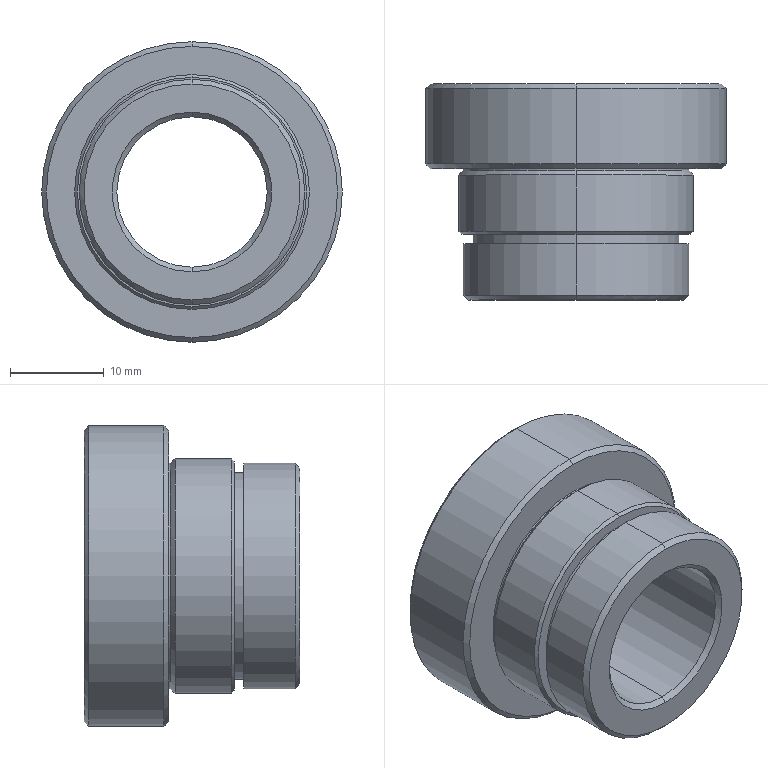Part | SolidWorks | features HoleWzd 1, Revolution 1 | 1 solid | 55 faces | box 32 x 23 x 32 mm | volume 8933 mm3 | cone 30 | cylinder 20 | plane 5 | commonest cylinder face diameters 2.5 x8 24 x4 16 x2 22 x2 25 x2 32 x2
STEP:
#1=CARTESIAN_POINT('',(-12.,-0.275,-1.25));
#2=VERTEX_POINT('',#1);
#3=CARTESIAN_POINT('',(-12.,-0.275,1.25));
#4=VERTEX_POINT('',#3);
#5=CARTESIAN_POINT('',(-12.,-0.275,0.));
#6=DIRECTION('',(0.,1.,0.));
#7=DIRECTION('',(0.,0.,1.));
#8=AXIS2_PLACEMENT_3D('',#5,#6,#7);
#9=CIRCLE('',#8,1.25);
#10=EDGE_CURVE('',#2,#4,#9,.T.);
#11=ORIENTED_EDGE('',*,*,#10,.F.);
#12=CARTESIAN_POINT('',(-12.,0.,-1.525));
#13=VERTEX_POINT('',#12);
#14=CARTESIAN_POINT('',(-12.,0.,-1.525));
#15=DIRECTION('',(0.,0.7071,-0.7071));
#16=VECTOR('',#15,1000.);
#17=LINE('',#14,#16);
#18=EDGE_CURVE('',#2,#13,#17,.T.);
#19=ORIENTED_EDGE('',*,*,#18,.T.);
#20=CARTESIAN_POINT('',(-12.,0.,1.525));
#21=VERTEX_POINT('',#20);
#22=CARTESIAN_POINT('',(-12.,0.,0.));
#23=DIRECTION('',(0.,1.,0.));
#24=DIRECTION('',(0.,0.,1.));
#25=AXIS2_PLACEMENT_3D('',#22,#23,#24);
#26=CIRCLE('',#25,1.525);
#27=EDGE_CURVE('',#13,#21,#26,.T.);
#28=ORIENTED_EDGE('',*,*,#27,.T.);
#29=CARTESIAN_POINT('',(-12.,0.,1.525));
#30=DIRECTION('',(0.,0.7071,0.7071));
#31=VECTOR('',#30,1000.);
#32=LINE('',#29,#31);
#33=EDGE_CURVE('',#4,#21,#32,.T.);
#34=ORIENTED_EDGE('',*,*,#33,.F.);
#35=EDGE_LOOP('',(#11,#19,#28,#34));
#36=FACE_OUTER_BOUND('',#35,.T.);
#37=CARTESIAN_POINT('',(-12.,0.,0.));
#38=DIRECTION('',(0.,1.,0.));
#39=DIRECTION('',(0.,0.,1.));
#40=AXIS2_PLACEMENT_3D('',#37,#38,#39);
#41=CONICAL_SURFACE('',#40,1.525,0.7854);
#42=ADVANCED_FACE('',(#36),#41,.F.);
#43=CARTESIAN_POINT('',(-12.,-7.,-1.25));
#44=VERTEX_POINT('',#43);
#45=CARTESIAN_POINT('',(-12.,-7.,1.25));
#46=VERTEX_POINT('',#45);
#47=CARTESIAN_POINT('',(-12.,-7.,0.));
#48=DIRECTION('',(0.,1.,0.));
#49=DIRECTION('',(0.,0.,1.));
#50=AXIS2_PLACEMENT_3D('',#47,#48,#49);
#51=CIRCLE('',#50,1.25);
#52=EDGE_CURVE('',#44,#46,#51,.T.);
#53=ORIENTED_EDGE('',*,*,#52,.F.);
#54=CARTESIAN_POINT('',(-12.,0.,-1.25));
#55=DIRECTION('',(0.,1.,0.));
#56=VECTOR('',#55,1000.);
#57=LINE('',#54,#56);
#58=EDGE_CURVE('',#44,#2,#57,.T.);
#59=ORIENTED_EDGE('',*,*,#58,.T.);
#60=ORIENTED_EDGE('',*,*,#10,.T.);
#61=CARTESIAN_POINT('',(-12.,0.,1.25));
#62=DIRECTION('',(0.,1.,0.));
#63=VECTOR('',#62,1000.);
#64=LINE('',#61,#63);
#65=EDGE_CURVE('',#46,#4,#64,.T.);
#66=ORIENTED_EDGE('',*,*,#65,.F.);
#67=EDGE_LOOP('',(#53,#59,#60,#66));
#68=FACE_OUTER_BOUND('',#67,.T.);
#69=CARTESIAN_POINT('',(-12.,0.,0.));
#70=DIRECTION('',(0.,1.,0.));
#71=DIRECTION('',(0.,0.,1.));
#72=AXIS2_PLACEMENT_3D('',#69,#70,#71);
#73=CYLINDRICAL_SURFACE('',#72,1.25);
#74=ADVANCED_FACE('',(#68),#73,.F.);
#75=CARTESIAN_POINT('',(-12.,-7.751,0.));
#76=VERTEX_POINT('',#75);
#77=CARTESIAN_POINT('',(-12.,-7.,1.25));
#78=DIRECTION('',(0.,0.515,0.8572));
#79=VECTOR('',#78,1000.);
#80=LINE('',#77,#79);
#81=EDGE_CURVE('',#76,#46,#80,.T.);
#82=ORIENTED_EDGE('',*,*,#81,.F.);
#83=CARTESIAN_POINT('',(-12.,-7.,-1.25));
#84=DIRECTION('',(0.,0.515,-0.8572));
#85=VECTOR('',#84,1000.);
#86=LINE('',#83,#85);
#87=EDGE_CURVE('',#76,#44,#86,.T.);
#88=ORIENTED_EDGE('',*,*,#87,.T.);
#89=ORIENTED_EDGE('',*,*,#52,.T.);
#90=EDGE_LOOP('',(#82,#88,#89));
#91=FACE_OUTER_BOUND('',#90,.T.);
#92=CARTESIAN_POINT('',(-12.,-7.,0.));
#93=DIRECTION('',(0.,1.,0.));
#94=DIRECTION('',(0.,0.,1.));
#95=AXIS2_PLACEMENT_3D('',#92,#93,#94);
#96=CONICAL_SURFACE('',#95,1.25,1.03);
#97=ADVANCED_FACE('',(#91),#96,.F.);
#98=CARTESIAN_POINT('',(0.,-0.275,-13.25));
#99=VERTEX_POINT('',#98);
#100=CARTESIAN_POINT('',(0.,-0.275,-10.75));
#101=VERTEX_POINT('',#100);
#102=CARTESIAN_POINT('',(0.,-0.275,-12.));
#103=DIRECTION('',(0.,1.,0.));
#104=DIRECTION('',(0.,0.,1.));
#105=AXIS2_PLACEMENT_3D('',#102,#103,#104);
#106=CIRCLE('',#105,1.25);
#107=EDGE_CURVE('',#99,#101,#106,.T.);
#108=ORIENTED_EDGE('',*,*,#107,.F.);
#109=CARTESIAN_POINT('',(0.,0.,-13.525));
#110=VERTEX_POINT('',#109);
#111=CARTESIAN_POINT('',(0.,0.,-13.525));
#112=DIRECTION('',(0.,0.7071,-0.7071));
#113=VECTOR('',#112,1000.);
#114=LINE('',#111,#113);
#115=EDGE_CURVE('',#99,#110,#114,.T.);
#116=ORIENTED_EDGE('',*,*,#115,.T.);
#117=CARTESIAN_POINT('',(0.,0.,-10.475));
#118=VERTEX_POINT('',#117);
#119=CARTESIAN_POINT('',(0.,0.,-12.));
#120=DIRECTION('',(0.,1.,0.));
#121=DIRECTION('',(0.,0.,1.));
#122=AXIS2_PLACEMENT_3D('',#119,#120,#121);
#123=CIRCLE('',#122,1.525);
#124=EDGE_CURVE('',#110,#118,#123,.T.);
#125=ORIENTED_EDGE('',*,*,#124,.T.);
#126=CARTESIAN_POINT('',(0.,0.,-10.475));
#127=DIRECTION('',(0.,0.7071,0.7071));
#128=VECTOR('',#127,1000.);
#129=LINE('',#126,#128);
#130=EDGE_CURVE('',#101,#118,#129,.T.);
#131=ORIENTED_EDGE('',*,*,#130,.F.);
#132=EDGE_LOOP('',(#108,#116,#125,#131));
#133=FACE_OUTER_BOUND('',#132,.T.);
#134=CARTESIAN_POINT('',(0.,0.,-12.));
#135=DIRECTION('',(0.,1.,0.));
#136=DIRECTION('',(0.,0.,1.));
#137=AXIS2_PLACEMENT_3D('',#134,#135,#136);
#138=CONICAL_SURFACE('',#137,1.525,0.7854);
#139=ADVANCED_FACE('',(#133),#138,.F.);
#140=CARTESIAN_POINT('',(0.,-7.,-13.25));
#141=VERTEX_POINT('',#140);
#142=CARTESIAN_POINT('',(0.,-7.,-10.75));
#143=VERTEX_POINT('',#142);
#144=CARTESIAN_POINT('',(0.,-7.,-12.));
#145=DIRECTION('',(0.,1.,0.));
#146=DIRECTION('',(0.,0.,1.));
#147=AXIS2_PLACEMENT_3D('',#144,#145,#146);
#148=CIRCLE('',#147,1.25);
#149=EDGE_CURVE('',#141,#143,#148,.T.);
#150=ORIENTED_EDGE('',*,*,#149,.F.);
#151=CARTESIAN_POINT('',(0.,0.,-13.25));
#152=DIRECTION('',(0.,1.,0.));
#153=VECTOR('',#152,1000.);
#154=LINE('',#151,#153);
#155=EDGE_CURVE('',#141,#99,#154,.T.);
#156=ORIENTED_EDGE('',*,*,#155,.T.);
#157=ORIENTED_EDGE('',*,*,#107,.T.);
#158=CARTESIAN_POINT('',(0.,0.,-10.75));
#159=DIRECTION('',(0.,1.,0.));
#160=VECTOR('',#159,1000.);
#161=LINE('',#158,#160);
#162=EDGE_CURVE('',#143,#101,#161,.T.);
#163=ORIENTED_EDGE('',*,*,#162,.F.);
#164=EDGE_LOOP('',(#150,#156,#157,#163));
#165=FACE_OUTER_BOUND('',#164,.T.);
#166=CARTESIAN_POINT('',(0.,0.,-12.));
#167=DIRECTION('',(0.,1.,0.));
#168=DIRECTION('',(0.,0.,1.));
#169=AXIS2_PLACEMENT_3D('',#166,#167,#168);
#170=CYLINDRICAL_SURFACE('',#169,1.25);
#171=ADVANCED_FACE('',(#165),#170,.F.);
#172=CARTESIAN_POINT('',(0.,-7.751,-12.));
#173=VERTEX_POINT('',#172);
#174=CARTESIAN_POINT('',(0.,-7.,-10.75));
#175=DIRECTION('',(0.,0.515,0.8572));
#176=VECTOR('',#175,1000.);
#177=LINE('',#174,#176);
#178=EDGE_CURVE('',#173,#143,#177,.T.);
#179=ORIENTED_EDGE('',*,*,#178,.F.);
#180=CARTESIAN_POINT('',(0.,-7.,-13.25));
#181=DIRECTION('',(0.,0.515,-0.8572));
#182=VECTOR('',#181,1000.);
#183=LINE('',#180,#182);
#184=EDGE_CURVE('',#173,#141,#183,.T.);
#185=ORIENTED_EDGE('',*,*,#184,.T.);
#186=ORIENTED_EDGE('',*,*,#149,.T.);
#187=EDGE_LOOP('',(#179,#185,#186));
#188=FACE_OUTER_BOUND('',#187,.T.);
#189=CARTESIAN_POINT('',(0.,-7.,-12.));
#190=DIRECTION('',(0.,1.,0.));
#191=DIRECTION('',(0.,0.,1.));
#192=AXIS2_PLACEMENT_3D('',#189,#190,#191);
#193=CONICAL_SURFACE('',#192,1.25,1.03);
#194=ADVANCED_FACE('',(#188),#193,.F.);
#195=CARTESIAN_POINT('',(12.,-0.275,-1.25));
#196=VERTEX_POINT('',#195);
#197=CARTESIAN_POINT('',(12.,-0.275,1.25));
#198=VERTEX_POINT('',#197);
#199=CARTESIAN_POINT('',(12.,-0.275,0.));
#200=DIRECTION('',(0.,1.,0.));
#201=DIRECTION('',(0.,0.,1.));
#202=AXIS2_PLACEMENT_3D('',#199,#200,#201);
#203=CIRCLE('',#202,1.25);
#204=EDGE_CURVE('',#196,#198,#203,.T.);
#205=ORIENTED_EDGE('',*,*,#204,.F.);
#206=CARTESIAN_POINT('',(12.,0.,-1.525));
#207=VERTEX_POINT('',#206);
#208=CARTESIAN_POINT('',(12.,0.,-1.525));
#209=DIRECTION('',(0.,0.7071,-0.7071));
#210=VECTOR('',#209,1000.);
#211=LINE('',#208,#210);
#212=EDGE_CURVE('',#196,#207,#211,.T.);
#213=ORIENTED_EDGE('',*,*,#212,.T.);
#214=CARTESIAN_POINT('',(12.,0.,1.525));
#215=VERTEX_POINT('',#214);
#216=CARTESIAN_POINT('',(12.,0.,0.));
#217=DIRECTION('',(0.,1.,0.));
#218=DIRECTION('',(0.,0.,1.));
#219=AXIS2_PLACEMENT_3D('',#216,#217,#218);
#220=CIRCLE('',#219,1.525);
#221=EDGE_CURVE('',#207,#215,#220,.T.);
#222=ORIENTED_EDGE('',*,*,#221,.T.);
#223=CARTESIAN_POINT('',(12.,0.,1.525));
#224=DIRECTION('',(0.,0.7071,0.7071));
#225=VECTOR('',#224,1000.);
#226=LINE('',#223,#225);
#227=EDGE_CURVE('',#198,#215,#226,.T.);
#228=ORIENTED_EDGE('',*,*,#227,.F.);
#229=EDGE_LOOP('',(#205,#213,#222,#228));
#230=FACE_OUTER_BOUND('',#229,.T.);
#231=CARTESIAN_POINT('',(12.,0.,0.));
#232=DIRECTION('',(0.,1.,0.));
#233=DIRECTION('',(0.,0.,1.));
#234=AXIS2_PLACEMENT_3D('',#231,#232,#233);
#235=CONICAL_SURFACE('',#234,1.525,0.7854);
#236=ADVANCED_FACE('',(#230),#235,.F.);
#237=CARTESIAN_POINT('',(12.,-7.,-1.25));
#238=VERTEX_POINT('',#237);
#239=CARTESIAN_POINT('',(12.,-7.,1.25));
#240=VERTEX_POINT('',#239);
#241=CARTESIAN_POINT('',(12.,-7.,0.));
#242=DIRECTION('',(0.,1.,0.));
#243=DIRECTION('',(0.,0.,1.));
#244=AXIS2_PLACEMENT_3D('',#241,#242,#243);
#245=CIRCLE('',#244,1.25);
#246=EDGE_CURVE('',#238,#240,#245,.T.);
#247=ORIENTED_EDGE('',*,*,#246,.F.);
#248=CARTESIAN_POINT('',(12.,0.,-1.25));
#249=DIRECTION('',(0.,1.,0.));
#250=VECTOR('',#249,1000.);
#251=LINE('',#248,#250);
#252=EDGE_CURVE('',#238,#196,#251,.T.);
#253=ORIENTED_EDGE('',*,*,#252,.T.);
#254=ORIENTED_EDGE('',*,*,#204,.T.);
#255=CARTESIAN_POINT('',(12.,0.,1.25));
#256=DIRECTION('',(0.,1.,0.));
#257=VECTOR('',#256,1000.);
#258=LINE('',#255,#257);
#259=EDGE_CURVE('',#240,#198,#258,.T.);
#260=ORIENTED_EDGE('',*,*,#259,.F.);
#261=EDGE_LOOP('',(#247,#253,#254,#260));
#262=FACE_OUTER_BOUND('',#261,.T.);
#263=CARTESIAN_POINT('',(12.,0.,0.));
#264=DIRECTION('',(0.,1.,0.));
#265=DIRECTION('',(0.,0.,1.));
#266=AXIS2_PLACEMENT_3D('',#263,#264,#265);
#267=CYLINDRICAL_SURFACE('',#266,1.25);
#268=ADVANCED_FACE('',(#262),#267,.F.);
#269=CARTESIAN_POINT('',(12.,-7.751,0.));
#270=VERTEX_POINT('',#269);
#271=CARTESIAN_POINT('',(12.,-7.,1.25));
#272=DIRECTION('',(0.,0.515,0.8572));
#273=VECTOR('',#272,1000.);
#274=LINE('',#271,#273);
#275=EDGE_CURVE('',#270,#240,#274,.T.);
#276=ORIENTED_EDGE('',*,*,#275,.F.);
#277=CARTESIAN_POINT('',(12.,-7.,-1.25));
#278=DIRECTION('',(0.,0.515,-0.8572));
#279=VECTOR('',#278,1000.);
#280=LINE('',#277,#279);
#281=EDGE_CURVE('',#270,#238,#280,.T.);
#282=ORIENTED_EDGE('',*,*,#281,.T.);
#283=ORIENTED_EDGE('',*,*,#246,.T.);
#284=EDGE_LOOP('',(#276,#282,#283));
#285=FACE_OUTER_BOUND('',#284,.T.);
#286=CARTESIAN_POINT('',(12.,-7.,0.));
#287=DIRECTION('',(0.,1.,0.));
#288=DIRECTION('',(0.,0.,1.));
#289=AXIS2_PLACEMENT_3D('',#286,#287,#288);
#290=CONICAL_SURFACE('',#289,1.25,1.03);
#291=ADVANCED_FACE('',(#285),#290,.F.);
#292=CARTESIAN_POINT('',(0.,-0.275,10.75));
#293=VERTEX_POINT('',#292);
#294=CARTESIAN_POINT('',(0.,-0.275,13.25));
#295=VERTEX_POINT('',#294);
#296=CARTESIAN_POINT('',(0.,-0.275,12.));
#297=DIRECTION('',(0.,1.,0.));
#298=DIRECTION('',(0.,0.,1.));
#299=AXIS2_PLACEMENT_3D('',#296,#297,#298);
#300=CIRCLE('',#299,1.25);
#301=EDGE_CURVE('',#293,#295,#300,.T.);
#302=ORIENTED_EDGE('',*,*,#301,.F.);
#303=CARTESIAN_POINT('',(0.,0.,10.475));
#304=VERTEX_POINT('',#303);
#305=CARTESIAN_POINT('',(0.,0.,10.475));
#306=DIRECTION('',(0.,0.7071,-0.7071));
#307=VECTOR('',#306,1000.);
#308=LINE('',#305,#307);
#309=EDGE_CURVE('',#293,#304,#308,.T.);
#310=ORIENTED_EDGE('',*,*,#309,.T.);
#311=CARTESIAN_POINT('',(0.,0.,13.525));
#312=VERTEX_POINT('',#311);
#313=CARTESIAN_POINT('',(0.,0.,12.));
#314=DIRECTION('',(0.,1.,0.));
#315=DIRECTION('',(0.,0.,1.));
#316=AXIS2_PLACEMENT_3D('',#313,#314,#315);
#317=CIRCLE('',#316,1.525);
#318=EDGE_CURVE('',#304,#312,#317,.T.);
#319=ORIENTED_EDGE('',*,*,#318,.T.);
#320=CARTESIAN_POINT('',(0.,0.,13.525));
#321=DIRECTION('',(0.,0.7071,0.7071));
#322=VECTOR('',#321,1000.);
#323=LINE('',#320,#322);
#324=EDGE_CURVE('',#295,#312,#323,.T.);
#325=ORIENTED_EDGE('',*,*,#324,.F.);
#326=EDGE_LOOP('',(#302,#310,#319,#325));
#327=FACE_OUTER_BOUND('',#326,.T.);
#328=CARTESIAN_POINT('',(0.,0.,12.));
#329=DIRECTION('',(0.,1.,0.));
#330=DIRECTION('',(0.,0.,1.));
#331=AXIS2_PLACEMENT_3D('',#328,#329,#330);
#332=CONICAL_SURFACE('',#331,1.525,0.7854);
#333=ADVANCED_FACE('',(#327),#332,.F.);
#334=CARTESIAN_POINT('',(0.,-7.,10.75));
#335=VERTEX_POINT('',#334);
#336=CARTESIAN_POINT('',(0.,-7.,13.25));
#337=VERTEX_POINT('',#336);
#338=CARTESIAN_POINT('',(0.,-7.,12.));
#339=DIRECTION('',(0.,1.,0.));
#340=DIRECTION('',(0.,0.,1.));
#341=AXIS2_PLACEMENT_3D('',#338,#339,#340);
#342=CIRCLE('',#341,1.25);
#343=EDGE_CURVE('',#335,#337,#342,.T.);
#344=ORIENTED_EDGE('',*,*,#343,.F.);
#345=CARTESIAN_POINT('',(0.,0.,10.75));
#346=DIRECTION('',(0.,1.,0.));
#347=VECTOR('',#346,1000.);
#348=LINE('',#345,#347);
#349=EDGE_CURVE('',#335,#293,#348,.T.);
#350=ORIENTED_EDGE('',*,*,#349,.T.);
#351=ORIENTED_EDGE('',*,*,#301,.T.);
#352=CARTESIAN_POINT('',(0.,0.,13.25));
#353=DIRECTION('',(0.,1.,0.));
#354=VECTOR('',#353,1000.);
#355=LINE('',#352,#354);
#356=EDGE_CURVE('',#337,#295,#355,.T.);
#357=ORIENTED_EDGE('',*,*,#356,.F.);
#358=EDGE_LOOP('',(#344,#350,#351,#357));
#359=FACE_OUTER_BOUND('',#358,.T.);
#360=CARTESIAN_POINT('',(0.,0.,12.));
#361=DIRECTION('',(0.,1.,0.));
#362=DIRECTION('',(0.,0.,1.));
#363=AXIS2_PLACEMENT_3D('',#360,#361,#362);
#364=CYLINDRICAL_SURFACE('',#363,1.25);
#365=ADVANCED_FACE('',(#359),#364,.F.);
#366=CARTESIAN_POINT('',(0.,-7.751,12.));
#367=VERTEX_POINT('',#366);
#368=CARTESIAN_POINT('',(0.,-7.,13.25));
#369=DIRECTION('',(0.,0.515,0.8572));
#370=VECTOR('',#369,1000.);
#371=LINE('',#368,#370);
#372=EDGE_CURVE('',#367,#337,#371,.T.);
#373=ORIENTED_EDGE('',*,*,#372,.F.);
#374=CARTESIAN_POINT('',(0.,-7.,10.75));
#375=DIRECTION('',(0.,0.515,-0.8572));
#376=VECTOR('',#375,1000.);
#377=LINE('',#374,#376);
#378=EDGE_CURVE('',#367,#335,#377,.T.);
#379=ORIENTED_EDGE('',*,*,#378,.T.);
#380=ORIENTED_EDGE('',*,*,#343,.T.);
#381=EDGE_LOOP('',(#373,#379,#380));
#382=FACE_OUTER_BOUND('',#381,.T.);
#383=CARTESIAN_POINT('',(0.,-7.,12.));
#384=DIRECTION('',(0.,1.,0.));
#385=DIRECTION('',(0.,0.,1.));
#386=AXIS2_PLACEMENT_3D('',#383,#384,#385);
#387=CONICAL_SURFACE('',#386,1.25,1.03);
#388=ADVANCED_FACE('',(#382),#387,.F.);
#389=CARTESIAN_POINT('',(0.,-22.5,-8.));
#390=VERTEX_POINT('',#389);
#391=CARTESIAN_POINT('',(0.,-22.5,8.));
#392=VERTEX_POINT('',#391);
#393=CARTESIAN_POINT('',(0.,-22.5,0.));
#394=DIRECTION('',(0.,1.,0.));
#395=DIRECTION('',(0.,0.,1.));
#396=AXIS2_PLACEMENT_3D('',#393,#394,#395);
#397=CIRCLE('',#396,8.);
#398=EDGE_CURVE('',#390,#392,#397,.T.);
#399=ORIENTED_EDGE('',*,*,#398,.F.);
#400=CARTESIAN_POINT('',(0.,-0.5,-8.));
#401=VERTEX_POINT('',#400);
#402=CARTESIAN_POINT('',(0.,0.,-8.));
#403=DIRECTION('',(0.,1.,0.));
#404=VECTOR('',#403,1000.);
#405=LINE('',#402,#404);
#406=EDGE_CURVE('',#390,#401,#405,.T.);
#407=ORIENTED_EDGE('',*,*,#406,.T.);
#408=CARTESIAN_POINT('',(0.,-0.5,8.));
#409=VERTEX_POINT('',#408);
#410=CARTESIAN_POINT('',(0.,-0.5,0.));
#411=DIRECTION('',(0.,1.,0.));
#412=DIRECTION('',(0.,0.,1.));
#413=AXIS2_PLACEMENT_3D('',#410,#411,#412);
#414=CIRCLE('',#413,8.);
#415=EDGE_CURVE('',#401,#409,#414,.T.);
#416=ORIENTED_EDGE('',*,*,#415,.T.);
#417=CARTESIAN_POINT('',(0.,0.,8.));
#418=DIRECTION('',(0.,1.,0.));
#419=VECTOR('',#418,1000.);
#420=LINE('',#417,#419);
#421=EDGE_CURVE('',#392,#409,#420,.T.);
#422=ORIENTED_EDGE('',*,*,#421,.F.);
#423=EDGE_LOOP('',(#399,#407,#416,#422));
#424=FACE_OUTER_BOUND('',#423,.T.);
#425=CARTESIAN_POINT('',(0.,0.,0.));
#426=DIRECTION('',(0.,1.,0.));
#427=DIRECTION('',(0.,0.,1.));
#428=AXIS2_PLACEMENT_3D('',#425,#426,#427);
#429=CYLINDRICAL_SURFACE('',#428,8.);
#430=ADVANCED_FACE('',(#424),#429,.F.);
#431=ORIENTED_EDGE('',*,*,#415,.F.);
#432=CARTESIAN_POINT('',(0.,0.,-8.5));
#433=VERTEX_POINT('',#432);
#434=CARTESIAN_POINT('',(0.,0.,-8.5));
#435=DIRECTION('',(0.,0.7071,-0.7071));
#436=VECTOR('',#435,1000.);
#437=LINE('',#434,#436);
#438=EDGE_CURVE('',#401,#433,#437,.T.);
#439=ORIENTED_EDGE('',*,*,#438,.T.);
#440=CARTESIAN_POINT('',(0.,0.,8.5));
#441=VERTEX_POINT('',#440);
#442=CARTESIAN_POINT('',(0.,0.,0.));
#443=DIRECTION('',(0.,1.,0.));
#444=DIRECTION('',(0.,0.,1.));
#445=AXIS2_PLACEMENT_3D('',#442,#443,#444);
#446=CIRCLE('',#445,8.5);
#447=EDGE_CURVE('',#433,#441,#446,.T.);
#448=ORIENTED_EDGE('',*,*,#447,.T.);
#449=CARTESIAN_POINT('',(0.,0.,8.5));
#450=DIRECTION('',(0.,0.7071,0.7071));
#451=VECTOR('',#450,1000.);
#452=LINE('',#449,#451);
#453=EDGE_CURVE('',#409,#441,#452,.T.);
#454=ORIENTED_EDGE('',*,*,#453,.F.);
#455=EDGE_LOOP('',(#431,#439,#448,#454));
#456=FACE_OUTER_BOUND('',#455,.T.);
#457=CARTESIAN_POINT('',(0.,0.,0.));
#458=DIRECTION('',(0.,1.,0.));
#459=DIRECTION('',(0.,0.,1.));
#460=AXIS2_PLACEMENT_3D('',#457,#458,#459);
#461=CONICAL_SURFACE('',#460,8.5,0.7854);
#462=ADVANCED_FACE('',(#456),#461,.F.);
#463=CARTESIAN_POINT('',(0.,0.,15.5));
#464=VERTEX_POINT('',#463);
#465=CARTESIAN_POINT('',(0.,0.,-15.5));
#466=VERTEX_POINT('',#465);
#467=CARTESIAN_POINT('',(0.,0.,0.));
#468=DIRECTION('',(0.,1.,0.));
#469=DIRECTION('',(0.,0.,1.));
#470=AXIS2_PLACEMENT_3D('',#467,#468,#469);
#471=CIRCLE('',#470,15.5);
#472=EDGE_CURVE('',#464,#466,#471,.T.);
#473=ORIENTED_EDGE('',*,*,#472,.F.);
#474=CARTESIAN_POINT('',(0.,-0.5,16.));
#475=VERTEX_POINT('',#474);
#476=CARTESIAN_POINT('',(0.,-0.5,16.));
#477=DIRECTION('',(0.,-0.7071,0.7071));
#478=VECTOR('',#477,1000.);
#479=LINE('',#476,#478);
#480=EDGE_CURVE('',#464,#475,#479,.T.);
#481=ORIENTED_EDGE('',*,*,#480,.T.);
#482=CARTESIAN_POINT('',(0.,-0.5,-16.));
#483=VERTEX_POINT('',#482);
#484=CARTESIAN_POINT('',(0.,-0.5,0.));
#485=DIRECTION('',(0.,1.,0.));
#486=DIRECTION('',(0.,0.,1.));
#487=AXIS2_PLACEMENT_3D('',#484,#485,#486);
#488=CIRCLE('',#487,16.);
#489=EDGE_CURVE('',#475,#483,#488,.T.);
#490=ORIENTED_EDGE('',*,*,#489,.T.);
#491=CARTESIAN_POINT('',(0.,-0.5,-16.));
#492=DIRECTION('',(0.,-0.7071,-0.7071));
#493=VECTOR('',#492,1000.);
#494=LINE('',#491,#493);
#495=EDGE_CURVE('',#466,#483,#494,.T.);
#496=ORIENTED_EDGE('',*,*,#495,.F.);
#497=EDGE_LOOP('',(#473,#481,#490,#496));
#498=FACE_OUTER_BOUND('',#497,.T.);
#499=CARTESIAN_POINT('',(0.,-0.5,0.));
#500=DIRECTION('',(0.,-1.,0.));
#501=DIRECTION('',(0.,0.,-1.));
#502=AXIS2_PLACEMENT_3D('',#499,#500,#501);
#503=CONICAL_SURFACE('',#502,16.,0.7854);
#504=ADVANCED_FACE('',(#498),#503,.T.);
#505=CARTESIAN_POINT('',(0.,-8.5,16.));
#506=VERTEX_POINT('',#505);
#507=CARTESIAN_POINT('',(0.,-8.5,-16.));
#508=VERTEX_POINT('',#507);
#509=CARTESIAN_POINT('',(0.,-8.5,0.));
#510=DIRECTION('',(0.,1.,0.));
#511=DIRECTION('',(0.,0.,1.));
#512=AXIS2_PLACEMENT_3D('',#509,#510,#511);
#513=CIRCLE('',#512,16.);
#514=EDGE_CURVE('',#506,#508,#513,.T.);
#515=ORIENTED_EDGE('',*,*,#514,.T.);
#516=CARTESIAN_POINT('',(0.,0.,-16.));
#517=DIRECTION('',(0.,1.,0.));
#518=VECTOR('',#517,1000.);
#519=LINE('',#516,#518);
#520=EDGE_CURVE('',#508,#483,#519,.T.);
#521=ORIENTED_EDGE('',*,*,#520,.T.);
#522=ORIENTED_EDGE('',*,*,#489,.F.);
#523=CARTESIAN_POINT('',(0.,0.,16.));
#524=DIRECTION('',(0.,1.,0.));
#525=VECTOR('',#524,1000.);
#526=LINE('',#523,#525);
#527=EDGE_CURVE('',#506,#475,#526,.T.);
#528=ORIENTED_EDGE('',*,*,#527,.F.);
#529=EDGE_LOOP('',(#515,#521,#522,#528));
#530=FACE_OUTER_BOUND('',#529,.T.);
#531=CARTESIAN_POINT('',(0.,0.,0.));
#532=DIRECTION('',(0.,1.,0.));
#533=DIRECTION('',(0.,0.,1.));
#534=AXIS2_PLACEMENT_3D('',#531,#532,#533);
#535=CYLINDRICAL_SURFACE('',#534,16.);
#536=ADVANCED_FACE('',(#530),#535,.T.);
#537=CARTESIAN_POINT('',(0.,-9.,15.5));
#538=VERTEX_POINT('',#537);
#539=CARTESIAN_POINT('',(0.,-9.,-15.5));
#540=VERTEX_POINT('',#539);
#541=CARTESIAN_POINT('',(0.,-9.,0.));
#542=DIRECTION('',(0.,1.,0.));
#543=DIRECTION('',(0.,0.,1.));
#544=AXIS2_PLACEMENT_3D('',#541,#542,#543);
#545=CIRCLE('',#544,15.5);
#546=EDGE_CURVE('',#538,#540,#545,.T.);
#547=ORIENTED_EDGE('',*,*,#546,.T.);
#548=CARTESIAN_POINT('',(0.,-9.,-15.5));
#549=DIRECTION('',(0.,0.7071,-0.7071));
#550=VECTOR('',#549,1000.);
#551=LINE('',#548,#550);
#552=EDGE_CURVE('',#540,#508,#551,.T.);
#553=ORIENTED_EDGE('',*,*,#552,.T.);
#554=ORIENTED_EDGE('',*,*,#514,.F.);
#555=CARTESIAN_POINT('',(0.,-9.,15.5));
#556=DIRECTION('',(0.,0.7071,0.7071));
#557=VECTOR('',#556,1000.);
#558=LINE('',#555,#557);
#559=EDGE_CURVE('',#538,#506,#558,.T.);
#560=ORIENTED_EDGE('',*,*,#559,.F.);
#561=EDGE_LOOP('',(#547,#553,#554,#560));
#562=FACE_OUTER_BOUND('',#561,.T.);
#563=CARTESIAN_POINT('',(0.,-9.,0.));
#564=DIRECTION('',(0.,1.,0.));
#565=DIRECTION('',(0.,0.,1.));
#566=AXIS2_PLACEMENT_3D('',#563,#564,#565);
#567=CONICAL_SURFACE('',#566,15.5,0.7854);
#568=ADVANCED_FACE('',(#562),#567,.T.);
#569=CARTESIAN_POINT('',(0.,-9.2,12.));
#570=VERTEX_POINT('',#569);
#571=CARTESIAN_POINT('',(0.,-9.2,-12.));
#572=VERTEX_POINT('',#571);
#573=CARTESIAN_POINT('',(0.,-9.2,0.));
#574=DIRECTION('',(0.,1.,0.));
#575=DIRECTION('',(0.,0.,1.));
#576=AXIS2_PLACEMENT_3D('',#573,#574,#575);
#577=CIRCLE('',#576,12.);
#578=EDGE_CURVE('',#570,#572,#577,.T.);
#579=ORIENTED_EDGE('',*,*,#578,.T.);
#580=CARTESIAN_POINT('',(0.,-9.,-12.));
#581=VERTEX_POINT('',#580);
#582=CARTESIAN_POINT('',(0.,0.,-12.));
#583=DIRECTION('',(0.,1.,0.));
#584=VECTOR('',#583,1000.);
#585=LINE('',#582,#584);
#586=EDGE_CURVE('',#572,#581,#585,.T.);
#587=ORIENTED_EDGE('',*,*,#586,.T.);
#588=CARTESIAN_POINT('',(0.,-9.,12.));
#589=VERTEX_POINT('',#588);
#590=CARTESIAN_POINT('',(0.,-9.,0.));
#591=DIRECTION('',(0.,1.,0.));
#592=DIRECTION('',(0.,0.,1.));
#593=AXIS2_PLACEMENT_3D('',#590,#591,#592);
#594=CIRCLE('',#593,12.);
#595=EDGE_CURVE('',#589,#581,#594,.T.);
#596=ORIENTED_EDGE('',*,*,#595,.F.);
#597=CARTESIAN_POINT('',(0.,0.,12.));
#598=DIRECTION('',(0.,1.,0.));
#599=VECTOR('',#598,1000.);
#600=LINE('',#597,#599);
#601=EDGE_CURVE('',#570,#589,#600,.T.);
#602=ORIENTED_EDGE('',*,*,#601,.F.);
#603=EDGE_LOOP('',(#579,#587,#596,#602));
#604=FACE_OUTER_BOUND('',#603,.T.);
#605=CARTESIAN_POINT('',(0.,0.,0.));
#606=DIRECTION('',(0.,1.,0.));
#607=DIRECTION('',(0.,0.,1.));
#608=AXIS2_PLACEMENT_3D('',#605,#606,#607);
#609=CYLINDRICAL_SURFACE('',#608,12.);
#610=ADVANCED_FACE('',(#604),#609,.T.);
#611=ORIENTED_EDGE('',*,*,#578,.F.);
#612=CARTESIAN_POINT('',(0.,-9.7,12.5));
#613=VERTEX_POINT('',#612);
#614=CARTESIAN_POINT('',(0.,-9.7,12.5));
#615=DIRECTION('',(0.,-0.7071,0.7071));
#616=VECTOR('',#615,1000.);
#617=LINE('',#614,#616);
#618=EDGE_CURVE('',#570,#613,#617,.T.);
#619=ORIENTED_EDGE('',*,*,#618,.T.);
#620=CARTESIAN_POINT('',(0.,-9.7,-12.5));
#621=VERTEX_POINT('',#620);
#622=CARTESIAN_POINT('',(0.,-9.7,0.));
#623=DIRECTION('',(0.,1.,0.));
#624=DIRECTION('',(0.,0.,1.));
#625=AXIS2_PLACEMENT_3D('',#622,#623,#624);
#626=CIRCLE('',#625,12.5);
#627=EDGE_CURVE('',#613,#621,#626,.T.);
#628=ORIENTED_EDGE('',*,*,#627,.T.);
#629=CARTESIAN_POINT('',(0.,-9.7,-12.5));
#630=DIRECTION('',(0.,-0.7071,-0.7071));
#631=VECTOR('',#630,1000.);
#632=LINE('',#629,#631);
#633=EDGE_CURVE('',#572,#621,#632,.T.);
#634=ORIENTED_EDGE('',*,*,#633,.F.);
#635=EDGE_LOOP('',(#611,#619,#628,#634));
#636=FACE_OUTER_BOUND('',#635,.T.);
#637=CARTESIAN_POINT('',(0.,-9.7,0.));
#638=DIRECTION('',(0.,-1.,0.));
#639=DIRECTION('',(0.,0.,-1.));
#640=AXIS2_PLACEMENT_3D('',#637,#638,#639);
#641=CONICAL_SURFACE('',#640,12.5,0.7854);
#642=ADVANCED_FACE('',(#636),#641,.T.);
#643=CARTESIAN_POINT('',(0.,-15.7,12.5));
#644=VERTEX_POINT('',#643);
#645=CARTESIAN_POINT('',(0.,-15.7,-12.5));
#646=VERTEX_POINT('',#645);
#647=CARTESIAN_POINT('',(0.,-15.7,0.));
#648=DIRECTION('',(0.,1.,0.));
#649=DIRECTION('',(0.,0.,1.));
#650=AXIS2_PLACEMENT_3D('',#647,#648,#649);
#651=CIRCLE('',#650,12.5);
#652=EDGE_CURVE('',#644,#646,#651,.T.);
#653=ORIENTED_EDGE('',*,*,#652,.T.);
#654=CARTESIAN_POINT('',(0.,0.,-12.5));
#655=DIRECTION('',(0.,1.,0.));
#656=VECTOR('',#655,1000.);
#657=LINE('',#654,#656);
#658=EDGE_CURVE('',#646,#621,#657,.T.);
#659=ORIENTED_EDGE('',*,*,#658,.T.);
#660=ORIENTED_EDGE('',*,*,#627,.F.);
#661=CARTESIAN_POINT('',(0.,0.,12.5));
#662=DIRECTION('',(0.,1.,0.));
#663=VECTOR('',#662,1000.);
#664=LINE('',#661,#663);
#665=EDGE_CURVE('',#644,#613,#664,.T.);
#666=ORIENTED_EDGE('',*,*,#665,.F.);
#667=EDGE_LOOP('',(#653,#659,#660,#666));
#668=FACE_OUTER_BOUND('',#667,.T.);
#669=CARTESIAN_POINT('',(0.,0.,0.));
#670=DIRECTION('',(0.,1.,0.));
#671=DIRECTION('',(0.,0.,1.));
#672=AXIS2_PLACEMENT_3D('',#669,#670,#671);
#673=CYLINDRICAL_SURFACE('',#672,12.5);
#674=ADVANCED_FACE('',(#668),#673,.T.);
#675=CARTESIAN_POINT('',(0.,-16.,12.2));
#676=VERTEX_POINT('',#675);
#677=CARTESIAN_POINT('',(0.,-16.,-12.2));
#678=VERTEX_POINT('',#677);
#679=CARTESIAN_POINT('',(0.,-16.,0.));
#680=DIRECTION('',(0.,1.,0.));
#681=DIRECTION('',(0.,0.,1.));
#682=AXIS2_PLACEMENT_3D('',#679,#680,#681);
#683=CIRCLE('',#682,12.2);
#684=EDGE_CURVE('',#676,#678,#683,.T.);
#685=ORIENTED_EDGE('',*,*,#684,.T.);
#686=CARTESIAN_POINT('',(0.,-16.,-12.2));
#687=DIRECTION('',(0.,0.7071,-0.7071));
#688=VECTOR('',#687,1000.);
#689=LINE('',#686,#688);
#690=EDGE_CURVE('',#678,#646,#689,.T.);
#691=ORIENTED_EDGE('',*,*,#690,.T.);
#692=ORIENTED_EDGE('',*,*,#652,.F.);
#693=CARTESIAN_POINT('',(0.,-16.,12.2));
#694=DIRECTION('',(0.,0.7071,0.7071));
#695=VECTOR('',#694,1000.);
#696=LINE('',#693,#695);
#697=EDGE_CURVE('',#676,#644,#696,.T.);
#698=ORIENTED_EDGE('',*,*,#697,.F.);
#699=EDGE_LOOP('',(#685,#691,#692,#698));
#700=FACE_OUTER_BOUND('',#699,.T.);
#701=CARTESIAN_POINT('',(0.,-16.,0.));
#702=DIRECTION('',(0.,1.,0.));
#703=DIRECTION('',(0.,0.,1.));
#704=AXIS2_PLACEMENT_3D('',#701,#702,#703);
#705=CONICAL_SURFACE('',#704,12.2,0.7854);
#706=ADVANCED_FACE('',(#700),#705,.T.);
#707=CARTESIAN_POINT('',(0.,-17.,11.));
#708=VERTEX_POINT('',#707);
#709=CARTESIAN_POINT('',(0.,-17.,-11.));
#710=VERTEX_POINT('',#709);
#711=CARTESIAN_POINT('',(0.,-17.,0.));
#712=DIRECTION('',(0.,1.,0.));
#713=DIRECTION('',(0.,0.,1.));
#714=AXIS2_PLACEMENT_3D('',#711,#712,#713);
#715=CIRCLE('',#714,11.);
#716=EDGE_CURVE('',#708,#710,#715,.T.);
#717=ORIENTED_EDGE('',*,*,#716,.T.);
#718=CARTESIAN_POINT('',(0.,-16.,-11.));
#719=VERTEX_POINT('',#718);
#720=CARTESIAN_POINT('',(0.,0.,-11.));
#721=DIRECTION('',(0.,1.,0.));
#722=VECTOR('',#721,1000.);
#723=LINE('',#720,#722);
#724=EDGE_CURVE('',#710,#719,#723,.T.);
#725=ORIENTED_EDGE('',*,*,#724,.T.);
#726=CARTESIAN_POINT('',(0.,-16.,11.));
#727=VERTEX_POINT('',#726);
#728=CARTESIAN_POINT('',(0.,-16.,0.));
#729=DIRECTION('',(0.,1.,0.));
#730=DIRECTION('',(0.,0.,1.));
#731=AXIS2_PLACEMENT_3D('',#728,#729,#730);
#732=CIRCLE('',#731,11.);
#733=EDGE_CURVE('',#727,#719,#732,.T.);
#734=ORIENTED_EDGE('',*,*,#733,.F.);
#735=CARTESIAN_POINT('',(0.,0.,11.));
#736=DIRECTION('',(0.,1.,0.));
#737=VECTOR('',#736,1000.);
#738=LINE('',#735,#737);
#739=EDGE_CURVE('',#708,#727,#738,.T.);
#740=ORIENTED_EDGE('',*,*,#739,.F.);
#741=EDGE_LOOP('',(#717,#725,#734,#740));
#742=FACE_OUTER_BOUND('',#741,.T.);
#743=CARTESIAN_POINT('',(0.,0.,0.));
#744=DIRECTION('',(0.,1.,0.));
#745=DIRECTION('',(0.,0.,1.));
#746=AXIS2_PLACEMENT_3D('',#743,#744,#745);
#747=CYLINDRICAL_SURFACE('',#746,11.);
#748=ADVANCED_FACE('',(#742),#747,.T.);
#749=CARTESIAN_POINT('',(0.,-22.5,12.));
#750=VERTEX_POINT('',#749);
#751=CARTESIAN_POINT('',(0.,-22.5,-12.));
#752=VERTEX_POINT('',#751);
#753=CARTESIAN_POINT('',(0.,-22.5,0.));
#754=DIRECTION('',(0.,1.,0.));
#755=DIRECTION('',(0.,0.,1.));
#756=AXIS2_PLACEMENT_3D('',#753,#754,#755);
#757=CIRCLE('',#756,12.);
#758=EDGE_CURVE('',#750,#752,#757,.T.);
#759=ORIENTED_EDGE('',*,*,#758,.T.);
#760=CARTESIAN_POINT('',(0.,-17.,-12.));
#761=VERTEX_POINT('',#760);
#762=CARTESIAN_POINT('',(0.,0.,-12.));
#763=DIRECTION('',(0.,1.,0.));
#764=VECTOR('',#763,1000.);
#765=LINE('',#762,#764);
#766=EDGE_CURVE('',#752,#761,#765,.T.);
#767=ORIENTED_EDGE('',*,*,#766,.T.);
#768=CARTESIAN_POINT('',(0.,-17.,12.));
#769=VERTEX_POINT('',#768);
#770=CARTESIAN_POINT('',(0.,-17.,0.));
#771=DIRECTION('',(0.,1.,0.));
#772=DIRECTION('',(0.,0.,1.));
#773=AXIS2_PLACEMENT_3D('',#770,#771,#772);
#774=CIRCLE('',#773,12.);
#775=EDGE_CURVE('',#769,#761,#774,.T.);
#776=ORIENTED_EDGE('',*,*,#775,.F.);
#777=CARTESIAN_POINT('',(0.,0.,12.));
#778=DIRECTION('',(0.,1.,0.));
#779=VECTOR('',#778,1000.);
#780=LINE('',#777,#779);
#781=EDGE_CURVE('',#750,#769,#780,.T.);
#782=ORIENTED_EDGE('',*,*,#781,.F.);
#783=EDGE_LOOP('',(#759,#767,#776,#782));
#784=FACE_OUTER_BOUND('',#783,.T.);
#785=CARTESIAN_POINT('',(0.,0.,0.));
#786=DIRECTION('',(0.,1.,0.));
#787=DIRECTION('',(0.,0.,1.));
#788=AXIS2_PLACEMENT_3D('',#785,#786,#787);
#789=CYLINDRICAL_SURFACE('',#788,12.);
#790=ADVANCED_FACE('',(#784),#789,.T.);
#791=CARTESIAN_POINT('',(0.,-23.,11.5));
#792=VERTEX_POINT('',#791);
#793=CARTESIAN_POINT('',(0.,-23.,-11.5));
#794=VERTEX_POINT('',#793);
#795=CARTESIAN_POINT('',(0.,-23.,0.));
#796=DIRECTION('',(0.,1.,0.));
#797=DIRECTION('',(0.,0.,1.));
#798=AXIS2_PLACEMENT_3D('',#795,#796,#797);
#799=CIRCLE('',#798,11.5);
#800=EDGE_CURVE('',#792,#794,#799,.T.);
#801=ORIENTED_EDGE('',*,*,#800,.T.);
#802=CARTESIAN_POINT('',(0.,-23.,-11.5));
#803=DIRECTION('',(0.,0.7071,-0.7071));
#804=VECTOR('',#803,1000.);
#805=LINE('',#802,#804);
#806=EDGE_CURVE('',#794,#752,#805,.T.);
#807=ORIENTED_EDGE('',*,*,#806,.T.);
#808=ORIENTED_EDGE('',*,*,#758,.F.);
#809=CARTESIAN_POINT('',(0.,-23.,11.5));
#810=DIRECTION('',(0.,0.7071,0.7071));
#811=VECTOR('',#810,1000.);
#812=LINE('',#809,#811);
#813=EDGE_CURVE('',#792,#750,#812,.T.);
#814=ORIENTED_EDGE('',*,*,#813,.F.);
#815=EDGE_LOOP('',(#801,#807,#808,#814));
#816=FACE_OUTER_BOUND('',#815,.T.);
#817=CARTESIAN_POINT('',(0.,-23.,0.));
#818=DIRECTION('',(0.,1.,0.));
#819=DIRECTION('',(0.,0.,1.));
#820=AXIS2_PLACEMENT_3D('',#817,#818,#819);
#821=CONICAL_SURFACE('',#820,11.5,0.7854);
#822=ADVANCED_FACE('',(#816),#821,.T.);
#823=ORIENTED_EDGE('',*,*,#398,.T.);
#824=CARTESIAN_POINT('',(0.,-23.,8.5));
#825=VERTEX_POINT('',#824);
#826=CARTESIAN_POINT('',(0.,-22.5,8.));
#827=DIRECTION('',(0.,-0.7071,0.7071));
#828=VECTOR('',#827,1000.);
#829=LINE('',#826,#828);
#830=EDGE_CURVE('',#392,#825,#829,.T.);
#831=ORIENTED_EDGE('',*,*,#830,.T.);
#832=CARTESIAN_POINT('',(0.,-23.,-8.5));
#833=VERTEX_POINT('',#832);
#834=CARTESIAN_POINT('',(0.,-23.,0.));
#835=DIRECTION('',(0.,1.,0.));
#836=DIRECTION('',(0.,0.,1.));
#837=AXIS2_PLACEMENT_3D('',#834,#835,#836);
#838=CIRCLE('',#837,8.5);
#839=EDGE_CURVE('',#833,#825,#838,.T.);
#840=ORIENTED_EDGE('',*,*,#839,.F.);
#841=CARTESIAN_POINT('',(0.,-22.5,-8.));
#842=DIRECTION('',(0.,-0.7071,-0.7071));
#843=VECTOR('',#842,1000.);
#844=LINE('',#841,#843);
#845=EDGE_CURVE('',#390,#833,#844,.T.);
#846=ORIENTED_EDGE('',*,*,#845,.F.);
#847=EDGE_LOOP('',(#823,#831,#840,#846));
#848=FACE_OUTER_BOUND('',#847,.T.);
#849=CARTESIAN_POINT('',(0.,-22.5,0.));
#850=DIRECTION('',(0.,-1.,0.));
#851=DIRECTION('',(0.,0.,-1.));
#852=AXIS2_PLACEMENT_3D('',#849,#850,#851);
#853=CONICAL_SURFACE('',#852,8.,0.7854);
#854=ADVANCED_FACE('',(#848),#853,.F.);
#855=ORIENTED_EDGE('',*,*,#830,.F.);
#856=CARTESIAN_POINT('',(0.,-22.5,0.));
#857=DIRECTION('',(0.,1.,0.));
#858=DIRECTION('',(0.,0.,1.));
#859=AXIS2_PLACEMENT_3D('',#856,#857,#858);
#860=CIRCLE('',#859,8.);
#861=EDGE_CURVE('',#392,#390,#860,.T.);
#862=ORIENTED_EDGE('',*,*,#861,.T.);
#863=ORIENTED_EDGE('',*,*,#845,.T.);
#864=CARTESIAN_POINT('',(0.,-23.,0.));
#865=DIRECTION('',(0.,1.,0.));
#866=DIRECTION('',(0.,0.,1.));
#867=AXIS2_PLACEMENT_3D('',#864,#865,#866);
#868=CIRCLE('',#867,8.5);
#869=EDGE_CURVE('',#825,#833,#868,.T.);
#870=ORIENTED_EDGE('',*,*,#869,.F.);
#871=EDGE_LOOP('',(#855,#862,#863,#870));
#872=FACE_OUTER_BOUND('',#871,.T.);
#873=CARTESIAN_POINT('',(0.,-22.5,0.));
#874=DIRECTION('',(0.,-1.,0.));
#875=DIRECTION('',(0.,0.,-1.));
#876=AXIS2_PLACEMENT_3D('',#873,#874,#875);
#877=CONICAL_SURFACE('',#876,8.,0.7854);
#878=ADVANCED_FACE('',(#872),#877,.F.);
#879=ORIENTED_EDGE('',*,*,#800,.F.);
#880=CARTESIAN_POINT('',(0.,-23.,0.));
#881=DIRECTION('',(0.,1.,0.));
#882=DIRECTION('',(0.,0.,1.));
#883=AXIS2_PLACEMENT_3D('',#880,#881,#882);
#884=CIRCLE('',#883,11.5);
#885=EDGE_CURVE('',#794,#792,#884,.T.);
#886=ORIENTED_EDGE('',*,*,#885,.F.);
#887=EDGE_LOOP('',(#879,#886));
#888=FACE_OUTER_BOUND('',#887,.T.);
#889=ORIENTED_EDGE('',*,*,#839,.T.);
#890=ORIENTED_EDGE('',*,*,#869,.T.);
#891=EDGE_LOOP('',(#889,#890));
#892=FACE_BOUND('',#891,.T.);
#893=CARTESIAN_POINT('',(8.5,-23.,0.));
#894=DIRECTION('',(0.,1.,0.));
#895=DIRECTION('',(0.,0.,1.));
#896=AXIS2_PLACEMENT_3D('',#893,#894,#895);
#897=PLANE('',#896);
#898=ADVANCED_FACE('',(#888,#892),#897,.F.);
#899=ORIENTED_EDGE('',*,*,#806,.F.);
#900=ORIENTED_EDGE('',*,*,#885,.T.);
#901=ORIENTED_EDGE('',*,*,#813,.T.);
#902=CARTESIAN_POINT('',(0.,-22.5,0.));
#903=DIRECTION('',(0.,1.,0.));
#904=DIRECTION('',(0.,0.,1.));
#905=AXIS2_PLACEMENT_3D('',#902,#903,#904);
#906=CIRCLE('',#905,12.);
#907=EDGE_CURVE('',#752,#750,#906,.T.);
#908=ORIENTED_EDGE('',*,*,#907,.F.);
#909=EDGE_LOOP('',(#899,#900,#901,#908));
#910=FACE_OUTER_BOUND('',#909,.T.);
#911=CARTESIAN_POINT('',(0.,-23.,0.));
#912=DIRECTION('',(0.,1.,0.));
#913=DIRECTION('',(0.,0.,1.));
#914=AXIS2_PLACEMENT_3D('',#911,#912,#913);
#915=CONICAL_SURFACE('',#914,11.5,0.7854);
#916=ADVANCED_FACE('',(#910),#915,.T.);
#917=ORIENTED_EDGE('',*,*,#766,.F.);
#918=ORIENTED_EDGE('',*,*,#907,.T.);
#919=ORIENTED_EDGE('',*,*,#781,.T.);
#920=CARTESIAN_POINT('',(0.,-17.,0.));
#921=DIRECTION('',(0.,1.,0.));
#922=DIRECTION('',(0.,0.,1.));
#923=AXIS2_PLACEMENT_3D('',#920,#921,#922);
#924=CIRCLE('',#923,12.);
#925=EDGE_CURVE('',#761,#769,#924,.T.);
#926=ORIENTED_EDGE('',*,*,#925,.F.);
#927=EDGE_LOOP('',(#917,#918,#919,#926));
#928=FACE_OUTER_BOUND('',#927,.T.);
#929=CARTESIAN_POINT('',(0.,0.,0.));
#930=DIRECTION('',(0.,1.,0.));
#931=DIRECTION('',(0.,0.,1.));
#932=AXIS2_PLACEMENT_3D('',#929,#930,#931);
#933=CYLINDRICAL_SURFACE('',#932,12.);
#934=ADVANCED_FACE('',(#928),#933,.T.);
#935=ORIENTED_EDGE('',*,*,#716,.F.);
#936=CARTESIAN_POINT('',(0.,-17.,0.));
#937=DIRECTION('',(0.,1.,0.));
#938=DIRECTION('',(0.,0.,1.));
#939=AXIS2_PLACEMENT_3D('',#936,#937,#938);
#940=CIRCLE('',#939,11.);
#941=EDGE_CURVE('',#710,#708,#940,.T.);
#942=ORIENTED_EDGE('',*,*,#941,.F.);
#943=EDGE_LOOP('',(#935,#942));
#944=FACE_BOUND('',#943,.T.);
#945=ORIENTED_EDGE('',*,*,#775,.T.);
#946=ORIENTED_EDGE('',*,*,#925,.T.);
#947=EDGE_LOOP('',(#945,#946));
#948=FACE_OUTER_BOUND('',#947,.T.);
#949=CARTESIAN_POINT('',(11.,-17.,0.));
#950=DIRECTION('',(0.,-1.,0.));
#951=DIRECTION('',(0.,0.,-1.));
#952=AXIS2_PLACEMENT_3D('',#949,#950,#951);
#953=PLANE('',#952);
#954=ADVANCED_FACE('',(#944,#948),#953,.F.);
#955=ORIENTED_EDGE('',*,*,#724,.F.);
#956=ORIENTED_EDGE('',*,*,#941,.T.);
#957=ORIENTED_EDGE('',*,*,#739,.T.);
#958=CARTESIAN_POINT('',(0.,-16.,0.));
#959=DIRECTION('',(0.,1.,0.));
#960=DIRECTION('',(0.,0.,1.));
#961=AXIS2_PLACEMENT_3D('',#958,#959,#960);
#962=CIRCLE('',#961,11.);
#963=EDGE_CURVE('',#719,#727,#962,.T.);
#964=ORIENTED_EDGE('',*,*,#963,.F.);
#965=EDGE_LOOP('',(#955,#956,#957,#964));
#966=FACE_OUTER_BOUND('',#965,.T.);
#967=CARTESIAN_POINT('',(0.,0.,0.));
#968=DIRECTION('',(0.,1.,0.));
#969=DIRECTION('',(0.,0.,1.));
#970=AXIS2_PLACEMENT_3D('',#967,#968,#969);
#971=CYLINDRICAL_SURFACE('',#970,11.);
#972=ADVANCED_FACE('',(#966),#971,.T.);
#973=ORIENTED_EDGE('',*,*,#684,.F.);
#974=CARTESIAN_POINT('',(0.,-16.,0.));
#975=DIRECTION('',(0.,1.,0.));
#976=DIRECTION('',(0.,0.,1.));
#977=AXIS2_PLACEMENT_3D('',#974,#975,#976);
#978=CIRCLE('',#977,12.2);
#979=EDGE_CURVE('',#678,#676,#978,.T.);
#980=ORIENTED_EDGE('',*,*,#979,.F.);
#981=EDGE_LOOP('',(#973,#980));
#982=FACE_OUTER_BOUND('',#981,.T.);
#983=ORIENTED_EDGE('',*,*,#733,.T.);
#984=ORIENTED_EDGE('',*,*,#963,.T.);
#985=EDGE_LOOP('',(#983,#984));
#986=FACE_BOUND('',#985,.T.);
#987=CARTESIAN_POINT('',(12.2,-16.,0.));
#988=DIRECTION('',(0.,1.,0.));
#989=DIRECTION('',(0.,0.,1.));
#990=AXIS2_PLACEMENT_3D('',#987,#988,#989);
#991=PLANE('',#990);
#992=ADVANCED_FACE('',(#982,#986),#991,.F.);
#993=ORIENTED_EDGE('',*,*,#690,.F.);
#994=ORIENTED_EDGE('',*,*,#979,.T.);
#995=ORIENTED_EDGE('',*,*,#697,.T.);
#996=CARTESIAN_POINT('',(0.,-15.7,0.));
#997=DIRECTION('',(0.,1.,0.));
#998=DIRECTION('',(0.,0.,1.));
#999=AXIS2_PLACEMENT_3D('',#996,#997,#998);
#1000=CIRCLE('',#999,12.5);
#1001=EDGE_CURVE('',#646,#644,#1000,.T.);
#1002=ORIENTED_EDGE('',*,*,#1001,.F.);
#1003=EDGE_LOOP('',(#993,#994,#995,#1002));
#1004=FACE_OUTER_BOUND('',#1003,.T.);
#1005=CARTESIAN_POINT('',(0.,-16.,0.));
#1006=DIRECTION('',(0.,1.,0.));
#1007=DIRECTION('',(0.,0.,1.));
#1008=AXIS2_PLACEMENT_3D('',#1005,#1006,#1007);
#1009=CONICAL_SURFACE('',#1008,12.2,0.7854);
#1010=ADVANCED_FACE('',(#1004),#1009,.T.);
#1011=ORIENTED_EDGE('',*,*,#658,.F.);
#1012=ORIENTED_EDGE('',*,*,#1001,.T.);
#1013=ORIENTED_EDGE('',*,*,#665,.T.);
#1014=CARTESIAN_POINT('',(0.,-9.7,0.));
#1015=DIRECTION('',(0.,1.,0.));
#1016=DIRECTION('',(0.,0.,1.));
#1017=AXIS2_PLACEMENT_3D('',#1014,#1015,#1016);
#1018=CIRCLE('',#1017,12.5);
#1019=EDGE_CURVE('',#621,#613,#1018,.T.);
#1020=ORIENTED_EDGE('',*,*,#1019,.F.);
#1021=EDGE_LOOP('',(#1011,#1012,#1013,#1020));
#1022=FACE_OUTER_BOUND('',#1021,.T.);
#1023=CARTESIAN_POINT('',(0.,0.,0.));
#1024=DIRECTION('',(0.,1.,0.));
#1025=DIRECTION('',(0.,0.,1.));
#1026=AXIS2_PLACEMENT_3D('',#1023,#1024,#1025);
#1027=CYLINDRICAL_SURFACE('',#1026,12.5);
#1028=ADVANCED_FACE('',(#1022),#1027,.T.);
#1029=ORIENTED_EDGE('',*,*,#618,.F.);
#1030=CARTESIAN_POINT('',(0.,-9.2,0.));
#1031=DIRECTION('',(0.,1.,0.));
#1032=DIRECTION('',(0.,0.,1.));
#1033=AXIS2_PLACEMENT_3D('',#1030,#1031,#1032);
#1034=CIRCLE('',#1033,12.);
#1035=EDGE_CURVE('',#572,#570,#1034,.T.);
#1036=ORIENTED_EDGE('',*,*,#1035,.F.);
#1037=ORIENTED_EDGE('',*,*,#633,.T.);
#1038=ORIENTED_EDGE('',*,*,#1019,.T.);
#1039=EDGE_LOOP('',(#1029,#1036,#1037,#1038));
#1040=FACE_OUTER_BOUND('',#1039,.T.);
#1041=CARTESIAN_POINT('',(0.,-9.7,0.));
#1042=DIRECTION('',(0.,-1.,0.));
#1043=DIRECTION('',(0.,0.,-1.));
#1044=AXIS2_PLACEMENT_3D('',#1041,#1042,#1043);
#1045=CONICAL_SURFACE('',#1044,12.5,0.7854);
#1046=ADVANCED_FACE('',(#1040),#1045,.T.);
#1047=ORIENTED_EDGE('',*,*,#586,.F.);
#1048=ORIENTED_EDGE('',*,*,#1035,.T.);
#1049=ORIENTED_EDGE('',*,*,#601,.T.);
#1050=CARTESIAN_POINT('',(0.,-9.,0.));
#1051=DIRECTION('',(0.,1.,0.));
#1052=DIRECTION('',(0.,0.,1.));
#1053=AXIS2_PLACEMENT_3D('',#1050,#1051,#1052);
#1054=CIRCLE('',#1053,12.);
#1055=EDGE_CURVE('',#581,#589,#1054,.T.);
#1056=ORIENTED_EDGE('',*,*,#1055,.F.);
#1057=EDGE_LOOP('',(#1047,#1048,#1049,#1056));
#1058=FACE_OUTER_BOUND('',#1057,.T.);
#1059=CARTESIAN_POINT('',(0.,0.,0.));
#1060=DIRECTION('',(0.,1.,0.));
#1061=DIRECTION('',(0.,0.,1.));
#1062=AXIS2_PLACEMENT_3D('',#1059,#1060,#1061);
#1063=CYLINDRICAL_SURFACE('',#1062,12.);
#1064=ADVANCED_FACE('',(#1058),#1063,.T.);
#1065=ORIENTED_EDGE('',*,*,#546,.F.);
#1066=CARTESIAN_POINT('',(0.,-9.,0.));
#1067=DIRECTION('',(0.,1.,0.));
#1068=DIRECTION('',(0.,0.,1.));
#1069=AXIS2_PLACEMENT_3D('',#1066,#1067,#1068);
#1070=CIRCLE('',#1069,15.5);
#1071=EDGE_CURVE('',#540,#538,#1070,.T.);
#1072=ORIENTED_EDGE('',*,*,#1071,.F.);
#1073=EDGE_LOOP('',(#1065,#1072));
#1074=FACE_OUTER_BOUND('',#1073,.T.);
#1075=ORIENTED_EDGE('',*,*,#595,.T.);
#1076=ORIENTED_EDGE('',*,*,#1055,.T.);
#1077=EDGE_LOOP('',(#1075,#1076));
#1078=FACE_BOUND('',#1077,.T.);
#1079=CARTESIAN_POINT('',(15.5,-9.,0.));
#1080=DIRECTION('',(0.,1.,0.));
#1081=DIRECTION('',(0.,0.,1.));
#1082=AXIS2_PLACEMENT_3D('',#1079,#1080,#1081);
#1083=PLANE('',#1082);
#1084=ADVANCED_FACE('',(#1074,#1078),#1083,.F.);
#1085=ORIENTED_EDGE('',*,*,#552,.F.);
#1086=ORIENTED_EDGE('',*,*,#1071,.T.);
#1087=ORIENTED_EDGE('',*,*,#559,.T.);
#1088=CARTESIAN_POINT('',(0.,-8.5,0.));
#1089=DIRECTION('',(0.,1.,0.));
#1090=DIRECTION('',(0.,0.,1.));
#1091=AXIS2_PLACEMENT_3D('',#1088,#1089,#1090);
#1092=CIRCLE('',#1091,16.);
#1093=EDGE_CURVE('',#508,#506,#1092,.T.);
#1094=ORIENTED_EDGE('',*,*,#1093,.F.);
#1095=EDGE_LOOP('',(#1085,#1086,#1087,#1094));
#1096=FACE_OUTER_BOUND('',#1095,.T.);
#1097=CARTESIAN_POINT('',(0.,-9.,0.));
#1098=DIRECTION('',(0.,1.,0.));
#1099=DIRECTION('',(0.,0.,1.));
#1100=AXIS2_PLACEMENT_3D('',#1097,#1098,#1099);
#1101=CONICAL_SURFACE('',#1100,15.5,0.7854);
#1102=ADVANCED_FACE('',(#1096),#1101,.T.);
#1103=ORIENTED_EDGE('',*,*,#520,.F.);
#1104=ORIENTED_EDGE('',*,*,#1093,.T.);
#1105=ORIENTED_EDGE('',*,*,#527,.T.);
#1106=CARTESIAN_POINT('',(0.,-0.5,0.));
#1107=DIRECTION('',(0.,1.,0.));
#1108=DIRECTION('',(0.,0.,1.));
#1109=AXIS2_PLACEMENT_3D('',#1106,#1107,#1108);
#1110=CIRCLE('',#1109,16.);
#1111=EDGE_CURVE('',#483,#475,#1110,.T.);
#1112=ORIENTED_EDGE('',*,*,#1111,.F.);
#1113=EDGE_LOOP('',(#1103,#1104,#1105,#1112));
#1114=FACE_OUTER_BOUND('',#1113,.T.);
#1115=CARTESIAN_POINT('',(0.,0.,0.));
#1116=DIRECTION('',(0.,1.,0.));
#1117=DIRECTION('',(0.,0.,1.));
#1118=AXIS2_PLACEMENT_3D('',#1115,#1116,#1117);
#1119=CYLINDRICAL_SURFACE('',#1118,16.);
#1120=ADVANCED_FACE('',(#1114),#1119,.T.);
#1121=ORIENTED_EDGE('',*,*,#480,.F.);
#1122=CARTESIAN_POINT('',(0.,0.,0.));
#1123=DIRECTION('',(0.,1.,0.));
#1124=DIRECTION('',(0.,0.,1.));
#1125=AXIS2_PLACEMENT_3D('',#1122,#1123,#1124);
#1126=CIRCLE('',#1125,15.5);
#1127=EDGE_CURVE('',#466,#464,#1126,.T.);
#1128=ORIENTED_EDGE('',*,*,#1127,.F.);
#1129=ORIENTED_EDGE('',*,*,#495,.T.);
#1130=ORIENTED_EDGE('',*,*,#1111,.T.);
#1131=EDGE_LOOP('',(#1121,#1128,#1129,#1130));
#1132=FACE_OUTER_BOUND('',#1131,.T.);
#1133=CARTESIAN_POINT('',(0.,-0.5,0.));
#1134=DIRECTION('',(0.,-1.,0.));
#1135=DIRECTION('',(0.,0.,-1.));
#1136=AXIS2_PLACEMENT_3D('',#1133,#1134,#1135);
#1137=CONICAL_SURFACE('',#1136,16.,0.7854);
#1138=ADVANCED_FACE('',(#1132),#1137,.T.);
#1139=CARTESIAN_POINT('',(-12.,0.,0.));
#1140=DIRECTION('',(0.,1.,0.));
#1141=DIRECTION('',(0.,0.,1.));
#1142=AXIS2_PLACEMENT_3D('',#1139,#1140,#1141);
#1143=CIRCLE('',#1142,1.525);
#1144=EDGE_CURVE('',#21,#13,#1143,.T.);
#1145=ORIENTED_EDGE('',*,*,#1144,.F.);
#1146=ORIENTED_EDGE('',*,*,#27,.F.);
#1147=EDGE_LOOP('',(#1145,#1146));
#1148=FACE_BOUND('',#1147,.T.);
#1149=CARTESIAN_POINT('',(0.,0.,-12.));
#1150=DIRECTION('',(0.,1.,0.));
#1151=DIRECTION('',(0.,0.,1.));
#1152=AXIS2_PLACEMENT_3D('',#1149,#1150,#1151);
#1153=CIRCLE('',#1152,1.525);
#1154=EDGE_CURVE('',#118,#110,#1153,.T.);
#1155=ORIENTED_EDGE('',*,*,#1154,.F.);
#1156=ORIENTED_EDGE('',*,*,#124,.F.);
#1157=EDGE_LOOP('',(#1155,#1156));
#1158=FACE_BOUND('',#1157,.T.);
#1159=CARTESIAN_POINT('',(12.,0.,0.));
#1160=DIRECTION('',(0.,1.,0.));
#1161=DIRECTION('',(0.,0.,1.));
#1162=AXIS2_PLACEMENT_3D('',#1159,#1160,#1161);
#1163=CIRCLE('',#1162,1.525);
#1164=EDGE_CURVE('',#215,#207,#1163,.T.);
#1165=ORIENTED_EDGE('',*,*,#1164,.F.);
#1166=ORIENTED_EDGE('',*,*,#221,.F.);
#1167=EDGE_LOOP('',(#1165,#1166));
#1168=FACE_BOUND('',#1167,.T.);
#1169=CARTESIAN_POINT('',(0.,0.,12.));
#1170=DIRECTION('',(0.,1.,0.));
#1171=DIRECTION('',(0.,0.,1.));
#1172=AXIS2_PLACEMENT_3D('',#1169,#1170,#1171);
#1173=CIRCLE('',#1172,1.525);
#1174=EDGE_CURVE('',#312,#304,#1173,.T.);
#1175=ORIENTED_EDGE('',*,*,#1174,.F.);
#1176=ORIENTED_EDGE('',*,*,#318,.F.);
#1177=EDGE_LOOP('',(#1175,#1176));
#1178=FACE_BOUND('',#1177,.T.);
#1179=CARTESIAN_POINT('',(0.,0.,0.));
#1180=DIRECTION('',(0.,1.,0.));
#1181=DIRECTION('',(0.,0.,1.));
#1182=AXIS2_PLACEMENT_3D('',#1179,#1180,#1181);
#1183=CIRCLE('',#1182,8.5);
#1184=EDGE_CURVE('',#441,#433,#1183,.T.);
#1185=ORIENTED_EDGE('',*,*,#1184,.F.);
#1186=ORIENTED_EDGE('',*,*,#447,.F.);
#1187=EDGE_LOOP('',(#1185,#1186));
#1188=FACE_BOUND('',#1187,.T.);
#1189=ORIENTED_EDGE('',*,*,#1127,.T.);
#1190=ORIENTED_EDGE('',*,*,#472,.T.);
#1191=EDGE_LOOP('',(#1189,#1190));
#1192=FACE_OUTER_BOUND('',#1191,.T.);
#1193=CARTESIAN_POINT('',(8.5,0.,0.));
#1194=DIRECTION('',(0.,-1.,0.));
#1195=DIRECTION('',(0.,0.,-1.));
#1196=AXIS2_PLACEMENT_3D('',#1193,#1194,#1195);
#1197=PLANE('',#1196);
#1198=ADVANCED_FACE('',(#1148,#1158,#1168,#1178,#1188,#1192),#1197,.F.);
#1199=ORIENTED_EDGE('',*,*,#438,.F.);
#1200=CARTESIAN_POINT('',(0.,-0.5,0.));
#1201=DIRECTION('',(0.,1.,0.));
#1202=DIRECTION('',(0.,0.,1.));
#1203=AXIS2_PLACEMENT_3D('',#1200,#1201,#1202);
#1204=CIRCLE('',#1203,8.);
#1205=EDGE_CURVE('',#409,#401,#1204,.T.);
#1206=ORIENTED_EDGE('',*,*,#1205,.F.);
#1207=ORIENTED_EDGE('',*,*,#453,.T.);
#1208=ORIENTED_EDGE('',*,*,#1184,.T.);
#1209=EDGE_LOOP('',(#1199,#1206,#1207,#1208));
#1210=FACE_OUTER_BOUND('',#1209,.T.);
#1211=CARTESIAN_POINT('',(0.,0.,0.));
#1212=DIRECTION('',(0.,1.,0.));
#1213=DIRECTION('',(0.,0.,1.));
#1214=AXIS2_PLACEMENT_3D('',#1211,#1212,#1213);
#1215=CONICAL_SURFACE('',#1214,8.5,0.7854);
#1216=ADVANCED_FACE('',(#1210),#1215,.F.);
#1217=ORIENTED_EDGE('',*,*,#406,.F.);
#1218=ORIENTED_EDGE('',*,*,#861,.F.);
#1219=ORIENTED_EDGE('',*,*,#421,.T.);
#1220=ORIENTED_EDGE('',*,*,#1205,.T.);
#1221=EDGE_LOOP('',(#1217,#1218,#1219,#1220));
#1222=FACE_OUTER_BOUND('',#1221,.T.);
#1223=CARTESIAN_POINT('',(0.,0.,0.));
#1224=DIRECTION('',(0.,1.,0.));
#1225=DIRECTION('',(0.,0.,1.));
#1226=AXIS2_PLACEMENT_3D('',#1223,#1224,#1225);
#1227=CYLINDRICAL_SURFACE('',#1226,8.);
#1228=ADVANCED_FACE('',(#1222),#1227,.F.);
#1229=ORIENTED_EDGE('',*,*,#378,.F.);
#1230=ORIENTED_EDGE('',*,*,#372,.T.);
#1231=CARTESIAN_POINT('',(0.,-7.,12.));
#1232=DIRECTION('',(0.,1.,0.));
#1233=DIRECTION('',(0.,0.,1.));
#1234=AXIS2_PLACEMENT_3D('',#1231,#1232,#1233);
#1235=CIRCLE('',#1234,1.25);
#1236=EDGE_CURVE('',#337,#335,#1235,.T.);
#1237=ORIENTED_EDGE('',*,*,#1236,.T.);
#1238=EDGE_LOOP('',(#1229,#1230,#1237));
#1239=FACE_OUTER_BOUND('',#1238,.T.);
#1240=CARTESIAN_POINT('',(0.,-7.,12.));
#1241=DIRECTION('',(0.,1.,0.));
#1242=DIRECTION('',(0.,0.,1.));
#1243=AXIS2_PLACEMENT_3D('',#1240,#1241,#1242);
#1244=CONICAL_SURFACE('',#1243,1.25,1.03);
#1245=ADVANCED_FACE('',(#1239),#1244,.F.);
#1246=ORIENTED_EDGE('',*,*,#349,.F.);
#1247=ORIENTED_EDGE('',*,*,#1236,.F.);
#1248=ORIENTED_EDGE('',*,*,#356,.T.);
#1249=CARTESIAN_POINT('',(0.,-0.275,12.));
#1250=DIRECTION('',(0.,1.,0.));
#1251=DIRECTION('',(0.,0.,1.));
#1252=AXIS2_PLACEMENT_3D('',#1249,#1250,#1251);
#1253=CIRCLE('',#1252,1.25);
#1254=EDGE_CURVE('',#295,#293,#1253,.T.);
#1255=ORIENTED_EDGE('',*,*,#1254,.T.);
#1256=EDGE_LOOP('',(#1246,#1247,#1248,#1255));
#1257=FACE_OUTER_BOUND('',#1256,.T.);
#1258=CARTESIAN_POINT('',(0.,0.,12.));
#1259=DIRECTION('',(0.,1.,0.));
#1260=DIRECTION('',(0.,0.,1.));
#1261=AXIS2_PLACEMENT_3D('',#1258,#1259,#1260);
#1262=CYLINDRICAL_SURFACE('',#1261,1.25);
#1263=ADVANCED_FACE('',(#1257),#1262,.F.);
#1264=ORIENTED_EDGE('',*,*,#309,.F.);
#1265=ORIENTED_EDGE('',*,*,#1254,.F.);
#1266=ORIENTED_EDGE('',*,*,#324,.T.);
#1267=ORIENTED_EDGE('',*,*,#1174,.T.);
#1268=EDGE_LOOP('',(#1264,#1265,#1266,#1267));
#1269=FACE_OUTER_BOUND('',#1268,.T.);
#1270=CARTESIAN_POINT('',(0.,0.,12.));
#1271=DIRECTION('',(0.,1.,0.));
#1272=DIRECTION('',(0.,0.,1.));
#1273=AXIS2_PLACEMENT_3D('',#1270,#1271,#1272);
#1274=CONICAL_SURFACE('',#1273,1.525,0.7854);
#1275=ADVANCED_FACE('',(#1269),#1274,.F.);
#1276=ORIENTED_EDGE('',*,*,#281,.F.);
#1277=ORIENTED_EDGE('',*,*,#275,.T.);
#1278=CARTESIAN_POINT('',(12.,-7.,0.));
#1279=DIRECTION('',(0.,1.,0.));
#1280=DIRECTION('',(0.,0.,1.));
#1281=AXIS2_PLACEMENT_3D('',#1278,#1279,#1280);
#1282=CIRCLE('',#1281,1.25);
#1283=EDGE_CURVE('',#240,#238,#1282,.T.);
#1284=ORIENTED_EDGE('',*,*,#1283,.T.);
#1285=EDGE_LOOP('',(#1276,#1277,#1284));
#1286=FACE_OUTER_BOUND('',#1285,.T.);
#1287=CARTESIAN_POINT('',(12.,-7.,0.));
#1288=DIRECTION('',(0.,1.,0.));
#1289=DIRECTION('',(0.,0.,1.));
#1290=AXIS2_PLACEMENT_3D('',#1287,#1288,#1289);
#1291=CONICAL_SURFACE('',#1290,1.25,1.03);
#1292=ADVANCED_FACE('',(#1286),#1291,.F.);
#1293=ORIENTED_EDGE('',*,*,#252,.F.);
#1294=ORIENTED_EDGE('',*,*,#1283,.F.);
#1295=ORIENTED_EDGE('',*,*,#259,.T.);
#1296=CARTESIAN_POINT('',(12.,-0.275,0.));
#1297=DIRECTION('',(0.,1.,0.));
#1298=DIRECTION('',(0.,0.,1.));
#1299=AXIS2_PLACEMENT_3D('',#1296,#1297,#1298);
#1300=CIRCLE('',#1299,1.25);
#1301=EDGE_CURVE('',#198,#196,#1300,.T.);
#1302=ORIENTED_EDGE('',*,*,#1301,.T.);
#1303=EDGE_LOOP('',(#1293,#1294,#1295,#1302));
#1304=FACE_OUTER_BOUND('',#1303,.T.);
#1305=CARTESIAN_POINT('',(12.,0.,0.));
#1306=DIRECTION('',(0.,1.,0.));
#1307=DIRECTION('',(0.,0.,1.));
#1308=AXIS2_PLACEMENT_3D('',#1305,#1306,#1307);
#1309=CYLINDRICAL_SURFACE('',#1308,1.25);
#1310=ADVANCED_FACE('',(#1304),#1309,.F.);
#1311=ORIENTED_EDGE('',*,*,#212,.F.);
#1312=ORIENTED_EDGE('',*,*,#1301,.F.);
#1313=ORIENTED_EDGE('',*,*,#227,.T.);
#1314=ORIENTED_EDGE('',*,*,#1164,.T.);
#1315=EDGE_LOOP('',(#1311,#1312,#1313,#1314));
#1316=FACE_OUTER_BOUND('',#1315,.T.);
#1317=CARTESIAN_POINT('',(12.,0.,0.));
#1318=DIRECTION('',(0.,1.,0.));
#1319=DIRECTION('',(0.,0.,1.));
#1320=AXIS2_PLACEMENT_3D('',#1317,#1318,#1319);
#1321=CONICAL_SURFACE('',#1320,1.525,0.7854);
#1322=ADVANCED_FACE('',(#1316),#1321,.F.);
#1323=ORIENTED_EDGE('',*,*,#184,.F.);
#1324=ORIENTED_EDGE('',*,*,#178,.T.);
#1325=CARTESIAN_POINT('',(0.,-7.,-12.));
#1326=DIRECTION('',(0.,1.,0.));
#1327=DIRECTION('',(0.,0.,1.));
#1328=AXIS2_PLACEMENT_3D('',#1325,#1326,#1327);
#1329=CIRCLE('',#1328,1.25);
#1330=EDGE_CURVE('',#143,#141,#1329,.T.);
#1331=ORIENTED_EDGE('',*,*,#1330,.T.);
#1332=EDGE_LOOP('',(#1323,#1324,#1331));
#1333=FACE_OUTER_BOUND('',#1332,.T.);
#1334=CARTESIAN_POINT('',(0.,-7.,-12.));
#1335=DIRECTION('',(0.,1.,0.));
#1336=DIRECTION('',(0.,0.,1.));
#1337=AXIS2_PLACEMENT_3D('',#1334,#1335,#1336);
#1338=CONICAL_SURFACE('',#1337,1.25,1.03);
#1339=ADVANCED_FACE('',(#1333),#1338,.F.);
#1340=ORIENTED_EDGE('',*,*,#155,.F.);
#1341=ORIENTED_EDGE('',*,*,#1330,.F.);
#1342=ORIENTED_EDGE('',*,*,#162,.T.);
#1343=CARTESIAN_POINT('',(0.,-0.275,-12.));
#1344=DIRECTION('',(0.,1.,0.));
#1345=DIRECTION('',(0.,0.,1.));
#1346=AXIS2_PLACEMENT_3D('',#1343,#1344,#1345);
#1347=CIRCLE('',#1346,1.25);
#1348=EDGE_CURVE('',#101,#99,#1347,.T.);
#1349=ORIENTED_EDGE('',*,*,#1348,.T.);
#1350=EDGE_LOOP('',(#1340,#1341,#1342,#1349));
#1351=FACE_OUTER_BOUND('',#1350,.T.);
#1352=CARTESIAN_POINT('',(0.,0.,-12.));
#1353=DIRECTION('',(0.,1.,0.));
#1354=DIRECTION('',(0.,0.,1.));
#1355=AXIS2_PLACEMENT_3D('',#1352,#1353,#1354);
#1356=CYLINDRICAL_SURFACE('',#1355,1.25);
#1357=ADVANCED_FACE('',(#1351),#1356,.F.);
#1358=ORIENTED_EDGE('',*,*,#115,.F.);
#1359=ORIENTED_EDGE('',*,*,#1348,.F.);
#1360=ORIENTED_EDGE('',*,*,#130,.T.);
#1361=ORIENTED_EDGE('',*,*,#1154,.T.);
#1362=EDGE_LOOP('',(#1358,#1359,#1360,#1361));
#1363=FACE_OUTER_BOUND('',#1362,.T.);
#1364=CARTESIAN_POINT('',(0.,0.,-12.));
#1365=DIRECTION('',(0.,1.,0.));
#1366=DIRECTION('',(0.,0.,1.));
#1367=AXIS2_PLACEMENT_3D('',#1364,#1365,#1366);
#1368=CONICAL_SURFACE('',#1367,1.525,0.7854);
#1369=ADVANCED_FACE('',(#1363),#1368,.F.);
#1370=ORIENTED_EDGE('',*,*,#87,.F.);
#1371=ORIENTED_EDGE('',*,*,#81,.T.);
#1372=CARTESIAN_POINT('',(-12.,-7.,0.));
#1373=DIRECTION('',(0.,1.,0.));
#1374=DIRECTION('',(0.,0.,1.));
#1375=AXIS2_PLACEMENT_3D('',#1372,#1373,#1374);
#1376=CIRCLE('',#1375,1.25);
#1377=EDGE_CURVE('',#46,#44,#1376,.T.);
#1378=ORIENTED_EDGE('',*,*,#1377,.T.);
#1379=EDGE_LOOP('',(#1370,#1371,#1378));
#1380=FACE_OUTER_BOUND('',#1379,.T.);
#1381=CARTESIAN_POINT('',(-12.,-7.,0.));
#1382=DIRECTION('',(0.,1.,0.));
#1383=DIRECTION('',(0.,0.,1.));
#1384=AXIS2_PLACEMENT_3D('',#1381,#1382,#1383);
#1385=CONICAL_SURFACE('',#1384,1.25,1.03);
#1386=ADVANCED_FACE('',(#1380),#1385,.F.);
#1387=ORIENTED_EDGE('',*,*,#58,.F.);
#1388=ORIENTED_EDGE('',*,*,#1377,.F.);
#1389=ORIENTED_EDGE('',*,*,#65,.T.);
#1390=CARTESIAN_POINT('',(-12.,-0.275,0.));
#1391=DIRECTION('',(0.,1.,0.));
#1392=DIRECTION('',(0.,0.,1.));
#1393=AXIS2_PLACEMENT_3D('',#1390,#1391,#1392);
#1394=CIRCLE('',#1393,1.25);
#1395=EDGE_CURVE('',#4,#2,#1394,.T.);
#1396=ORIENTED_EDGE('',*,*,#1395,.T.);
#1397=EDGE_LOOP('',(#1387,#1388,#1389,#1396));
#1398=FACE_OUTER_BOUND('',#1397,.T.);
#1399=CARTESIAN_POINT('',(-12.,0.,0.));
#1400=DIRECTION('',(0.,1.,0.));
#1401=DIRECTION('',(0.,0.,1.));
#1402=AXIS2_PLACEMENT_3D('',#1399,#1400,#1401);
#1403=CYLINDRICAL_SURFACE('',#1402,1.25);
#1404=ADVANCED_FACE('',(#1398),#1403,.F.);
#1405=ORIENTED_EDGE('',*,*,#18,.F.);
#1406=ORIENTED_EDGE('',*,*,#1395,.F.);
#1407=ORIENTED_EDGE('',*,*,#33,.T.);
#1408=ORIENTED_EDGE('',*,*,#1144,.T.);
#1409=EDGE_LOOP('',(#1405,#1406,#1407,#1408));
#1410=FACE_OUTER_BOUND('',#1409,.T.);
#1411=CARTESIAN_POINT('',(-12.,0.,0.));
#1412=DIRECTION('',(0.,1.,0.));
#1413=DIRECTION('',(0.,0.,1.));
#1414=AXIS2_PLACEMENT_3D('',#1411,#1412,#1413);
#1415=CONICAL_SURFACE('',#1414,1.525,0.7854);
#1416=ADVANCED_FACE('',(#1410),#1415,.F.);
#1417=CLOSED_SHELL('',(#42,#74,#97,#139,#171,#194,#236,#268,#291,#333,#365,#388,#430,#462,#504,#536,#568,#610,#642,#674,#706,#748,#790,#822,#854,#878,#898,#916,#934,#954,#972,#992,#1010,#1028,#1046,#1064,#1084,#1102,#1120,#1138,#1198,#1216,#1228,#1245,#1263,#1275,#1292,#1310,#1322,#1339,#1357,#1369,#1386,#1404,#1416));
#1418=MANIFOLD_SOLID_BREP('',#1417);
#1419=CARTESIAN_POINT('',(0.,0.,0.));
#1420=DIRECTION('',(0.,0.,1.));
#1421=DIRECTION('',(1.,0.,0.));
#1422=AXIS2_PLACEMENT_3D('',#1419,#1420,#1421);
#1423=(LENGTH_UNIT()NAMED_UNIT(*)SI_UNIT(.MILLI.,.METRE.));
#1424=UNCERTAINTY_MEASURE_WITH_UNIT(LENGTH_MEASURE(0.00001),#1423,'','');
#1425=(NAMED_UNIT(*)PLANE_ANGLE_UNIT()SI_UNIT($,.RADIAN.));
#1426=(NAMED_UNIT(*)SI_UNIT($,.STERADIAN.)SOLID_ANGLE_UNIT());
#1427=(GEOMETRIC_REPRESENTATION_CONTEXT(3)GLOBAL_UNCERTAINTY_ASSIGNED_CONTEXT((#1424))GLOBAL_UNIT_ASSIGNED_CONTEXT((#1423,#1425,#1426))REPRESENTATION_CONTEXT('',''));
#1428=ADVANCED_BREP_SHAPE_REPRESENTATION('',(#1418,#1422),#1427);